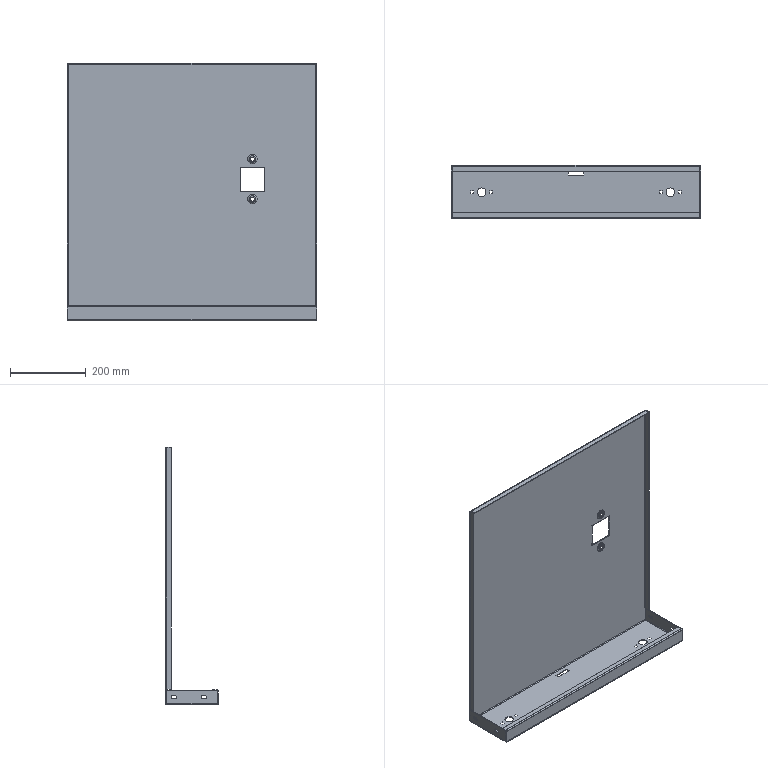Part | STEP file | 1 solid | 166 faces | box 660 x 140 x 682 mm | volume 1198837 mm3 | plane 106 | cylinder 44 | torus 16 | commonest cylinder face diameters 7 x20 3 x8 11 x4 20 x4 23 x4 24 x4